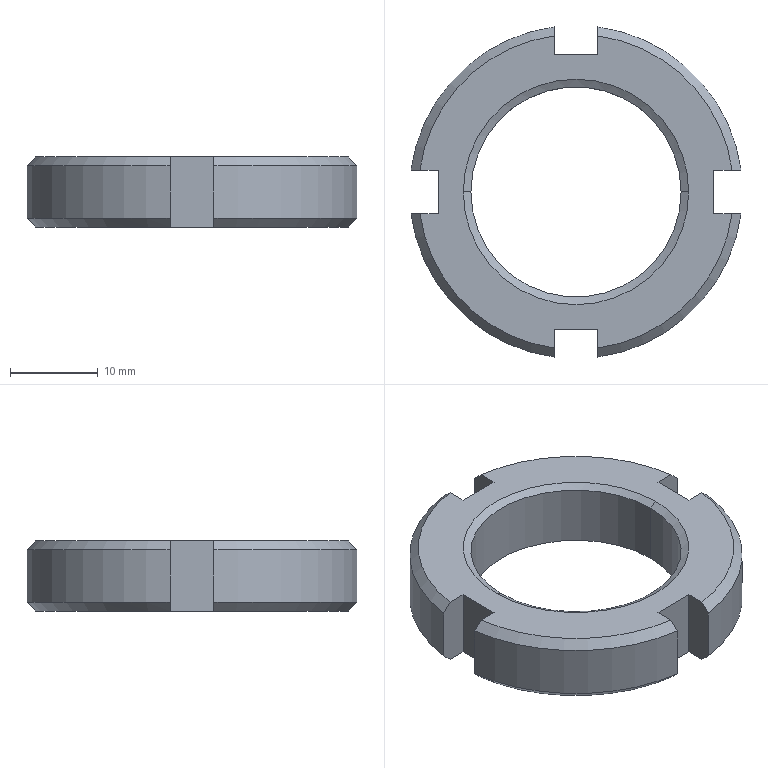Part | STEP file | Round Nut GB/T810-1988 M24x1.5 | 1 solid | 32 faces | box 37.67 x 37.67 x 8 mm | volume 4810 mm3 | plane 14 | cone 12 | cylinder 6 | commonest cylinder face diameters 38 x4 24 x2